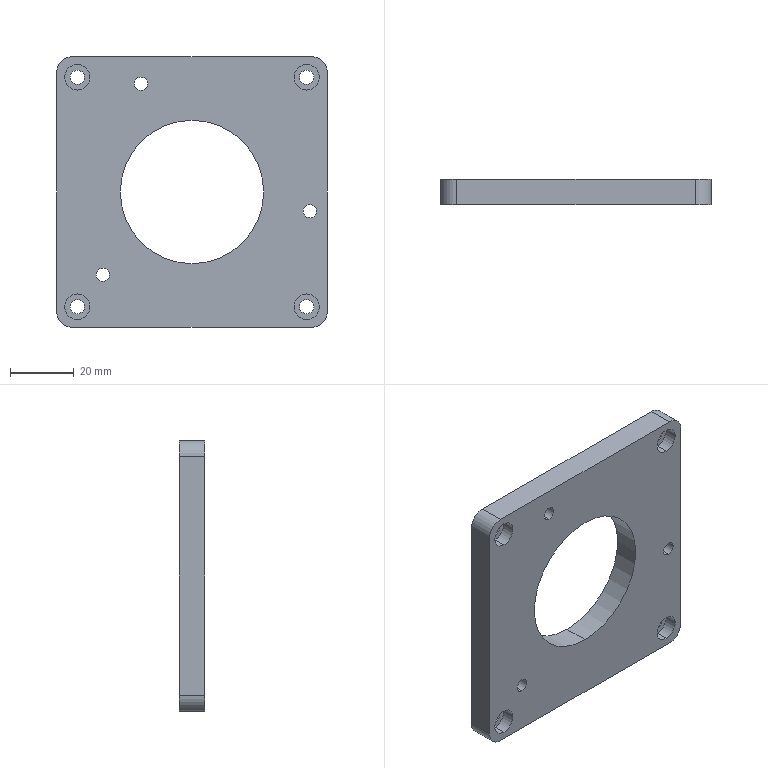Part | STEP file | 1 solid | 38 faces | box 85 x 8 x 85 mm | volume 43514 mm3 | cylinder 28 | plane 10 | commonest cylinder face diameters 4.5 x8 8 x8 4.2 x6 10 x4 45 x2